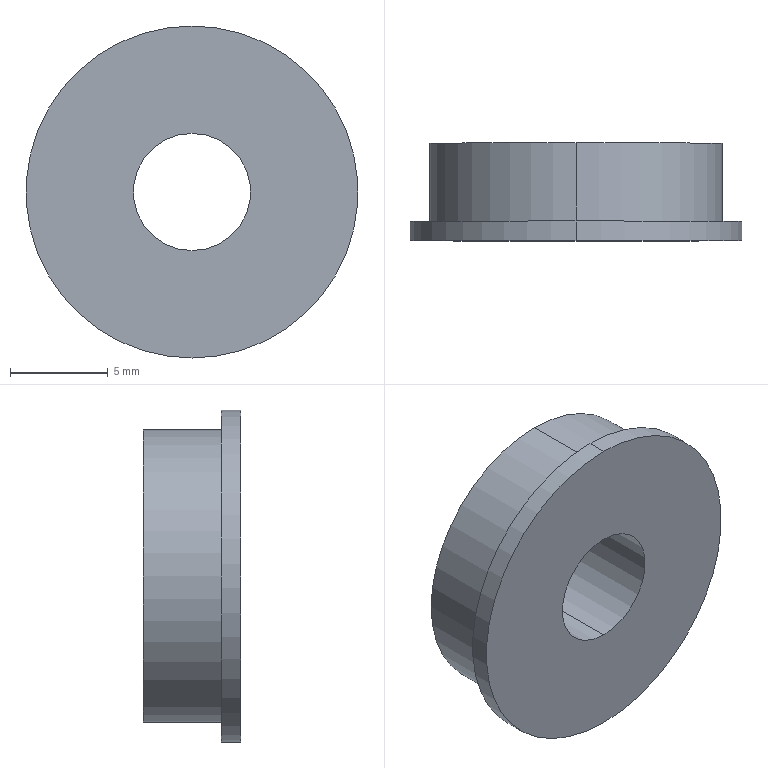Part | SolidWorks | features Revolution 1 | 1 solid | 9 faces | box 17 x 5 x 17 mm | volume 792.467 mm3 | cylinder 6 | plane 3 | commonest cylinder face diameters 6 x2 15 x2 17 x2
STEP:
#1=CARTESIAN_POINT('',(0.,-1.683,-8.5));
#2=VERTEX_POINT('',#1);
#3=CARTESIAN_POINT('',(0.,-1.683,8.5));
#4=VERTEX_POINT('',#3);
#5=CARTESIAN_POINT('',(0.,-1.683,0.));
#6=DIRECTION('',(0.,-1.,0.));
#7=DIRECTION('',(0.,0.,-1.));
#8=AXIS2_PLACEMENT_3D('',#5,#6,#7);
#9=CIRCLE('',#8,8.5);
#10=EDGE_CURVE('',#2,#4,#9,.T.);
#11=ORIENTED_EDGE('',*,*,#10,.T.);
#12=CARTESIAN_POINT('',(0.,-2.683,8.5));
#13=VERTEX_POINT('',#12);
#14=CARTESIAN_POINT('',(0.,0.,8.5));
#15=DIRECTION('',(0.,-1.,0.));
#16=VECTOR('',#15,1000.);
#17=LINE('',#14,#16);
#18=EDGE_CURVE('',#4,#13,#17,.T.);
#19=ORIENTED_EDGE('',*,*,#18,.T.);
#20=CARTESIAN_POINT('',(0.,-2.683,-8.5));
#21=VERTEX_POINT('',#20);
#22=CARTESIAN_POINT('',(0.,-2.683,0.));
#23=DIRECTION('',(0.,-1.,0.));
#24=DIRECTION('',(0.,0.,-1.));
#25=AXIS2_PLACEMENT_3D('',#22,#23,#24);
#26=CIRCLE('',#25,8.5);
#27=EDGE_CURVE('',#21,#13,#26,.T.);
#28=ORIENTED_EDGE('',*,*,#27,.F.);
#29=CARTESIAN_POINT('',(0.,0.,-8.5));
#30=DIRECTION('',(0.,-1.,0.));
#31=VECTOR('',#30,1000.);
#32=LINE('',#29,#31);
#33=EDGE_CURVE('',#2,#21,#32,.T.);
#34=ORIENTED_EDGE('',*,*,#33,.F.);
#35=EDGE_LOOP('',(#11,#19,#28,#34));
#36=FACE_OUTER_BOUND('',#35,.T.);
#37=CARTESIAN_POINT('',(0.,0.,0.));
#38=DIRECTION('',(0.,-1.,0.));
#39=DIRECTION('',(0.,0.,-1.));
#40=AXIS2_PLACEMENT_3D('',#37,#38,#39);
#41=CYLINDRICAL_SURFACE('',#40,8.5);
#42=ADVANCED_FACE('',(#36),#41,.T.);
#43=CARTESIAN_POINT('',(0.,2.317,-7.5));
#44=VERTEX_POINT('',#43);
#45=CARTESIAN_POINT('',(0.,2.317,7.5));
#46=VERTEX_POINT('',#45);
#47=CARTESIAN_POINT('',(0.,2.317,0.));
#48=DIRECTION('',(0.,-1.,0.));
#49=DIRECTION('',(0.,0.,-1.));
#50=AXIS2_PLACEMENT_3D('',#47,#48,#49);
#51=CIRCLE('',#50,7.5);
#52=EDGE_CURVE('',#44,#46,#51,.T.);
#53=ORIENTED_EDGE('',*,*,#52,.T.);
#54=CARTESIAN_POINT('',(0.,-1.683,7.5));
#55=VERTEX_POINT('',#54);
#56=CARTESIAN_POINT('',(0.,0.,7.5));
#57=DIRECTION('',(0.,-1.,0.));
#58=VECTOR('',#57,1000.);
#59=LINE('',#56,#58);
#60=EDGE_CURVE('',#46,#55,#59,.T.);
#61=ORIENTED_EDGE('',*,*,#60,.T.);
#62=CARTESIAN_POINT('',(0.,-1.683,-7.5));
#63=VERTEX_POINT('',#62);
#64=CARTESIAN_POINT('',(0.,-1.683,0.));
#65=DIRECTION('',(0.,-1.,0.));
#66=DIRECTION('',(0.,0.,-1.));
#67=AXIS2_PLACEMENT_3D('',#64,#65,#66);
#68=CIRCLE('',#67,7.5);
#69=EDGE_CURVE('',#63,#55,#68,.T.);
#70=ORIENTED_EDGE('',*,*,#69,.F.);
#71=CARTESIAN_POINT('',(0.,0.,-7.5));
#72=DIRECTION('',(0.,-1.,0.));
#73=VECTOR('',#72,1000.);
#74=LINE('',#71,#73);
#75=EDGE_CURVE('',#44,#63,#74,.T.);
#76=ORIENTED_EDGE('',*,*,#75,.F.);
#77=EDGE_LOOP('',(#53,#61,#70,#76));
#78=FACE_OUTER_BOUND('',#77,.T.);
#79=CARTESIAN_POINT('',(0.,0.,0.));
#80=DIRECTION('',(0.,-1.,0.));
#81=DIRECTION('',(0.,0.,-1.));
#82=AXIS2_PLACEMENT_3D('',#79,#80,#81);
#83=CYLINDRICAL_SURFACE('',#82,7.5);
#84=ADVANCED_FACE('',(#78),#83,.T.);
#85=CARTESIAN_POINT('',(0.,2.317,3.));
#86=VERTEX_POINT('',#85);
#87=CARTESIAN_POINT('',(0.,2.317,-3.));
#88=VERTEX_POINT('',#87);
#89=CARTESIAN_POINT('',(0.,2.317,0.));
#90=DIRECTION('',(0.,-1.,0.));
#91=DIRECTION('',(0.,0.,-1.));
#92=AXIS2_PLACEMENT_3D('',#89,#90,#91);
#93=CIRCLE('',#92,3.);
#94=EDGE_CURVE('',#86,#88,#93,.T.);
#95=ORIENTED_EDGE('',*,*,#94,.F.);
#96=CARTESIAN_POINT('',(0.,-2.683,3.));
#97=VERTEX_POINT('',#96);
#98=CARTESIAN_POINT('',(0.,0.,3.));
#99=DIRECTION('',(0.,-1.,0.));
#100=VECTOR('',#99,1000.);
#101=LINE('',#98,#100);
#102=EDGE_CURVE('',#86,#97,#101,.T.);
#103=ORIENTED_EDGE('',*,*,#102,.T.);
#104=CARTESIAN_POINT('',(0.,-2.683,-3.));
#105=VERTEX_POINT('',#104);
#106=CARTESIAN_POINT('',(0.,-2.683,0.));
#107=DIRECTION('',(0.,-1.,0.));
#108=DIRECTION('',(0.,0.,-1.));
#109=AXIS2_PLACEMENT_3D('',#106,#107,#108);
#110=CIRCLE('',#109,3.);
#111=EDGE_CURVE('',#97,#105,#110,.T.);
#112=ORIENTED_EDGE('',*,*,#111,.T.);
#113=CARTESIAN_POINT('',(0.,0.,-3.));
#114=DIRECTION('',(0.,-1.,0.));
#115=VECTOR('',#114,1000.);
#116=LINE('',#113,#115);
#117=EDGE_CURVE('',#88,#105,#116,.T.);
#118=ORIENTED_EDGE('',*,*,#117,.F.);
#119=EDGE_LOOP('',(#95,#103,#112,#118));
#120=FACE_OUTER_BOUND('',#119,.T.);
#121=CARTESIAN_POINT('',(0.,0.,0.));
#122=DIRECTION('',(0.,-1.,0.));
#123=DIRECTION('',(0.,0.,-1.));
#124=AXIS2_PLACEMENT_3D('',#121,#122,#123);
#125=CYLINDRICAL_SURFACE('',#124,3.);
#126=ADVANCED_FACE('',(#120),#125,.F.);
#127=ORIENTED_EDGE('',*,*,#102,.F.);
#128=CARTESIAN_POINT('',(0.,2.317,0.));
#129=DIRECTION('',(0.,-1.,0.));
#130=DIRECTION('',(0.,0.,-1.));
#131=AXIS2_PLACEMENT_3D('',#128,#129,#130);
#132=CIRCLE('',#131,3.);
#133=EDGE_CURVE('',#88,#86,#132,.T.);
#134=ORIENTED_EDGE('',*,*,#133,.F.);
#135=ORIENTED_EDGE('',*,*,#117,.T.);
#136=CARTESIAN_POINT('',(0.,-2.683,0.));
#137=DIRECTION('',(0.,-1.,0.));
#138=DIRECTION('',(0.,0.,-1.));
#139=AXIS2_PLACEMENT_3D('',#136,#137,#138);
#140=CIRCLE('',#139,3.);
#141=EDGE_CURVE('',#105,#97,#140,.T.);
#142=ORIENTED_EDGE('',*,*,#141,.T.);
#143=EDGE_LOOP('',(#127,#134,#135,#142));
#144=FACE_OUTER_BOUND('',#143,.T.);
#145=CARTESIAN_POINT('',(0.,0.,0.));
#146=DIRECTION('',(0.,-1.,0.));
#147=DIRECTION('',(0.,0.,-1.));
#148=AXIS2_PLACEMENT_3D('',#145,#146,#147);
#149=CYLINDRICAL_SURFACE('',#148,3.);
#150=ADVANCED_FACE('',(#144),#149,.F.);
#151=ORIENTED_EDGE('',*,*,#133,.T.);
#152=ORIENTED_EDGE('',*,*,#94,.T.);
#153=EDGE_LOOP('',(#151,#152));
#154=FACE_BOUND('',#153,.T.);
#155=ORIENTED_EDGE('',*,*,#52,.F.);
#156=CARTESIAN_POINT('',(0.,2.317,0.));
#157=DIRECTION('',(0.,-1.,0.));
#158=DIRECTION('',(0.,0.,-1.));
#159=AXIS2_PLACEMENT_3D('',#156,#157,#158);
#160=CIRCLE('',#159,7.5);
#161=EDGE_CURVE('',#46,#44,#160,.T.);
#162=ORIENTED_EDGE('',*,*,#161,.F.);
#163=EDGE_LOOP('',(#155,#162));
#164=FACE_OUTER_BOUND('',#163,.T.);
#165=CARTESIAN_POINT('',(3.,2.317,0.));
#166=DIRECTION('',(0.,1.,0.));
#167=DIRECTION('',(0.,0.,1.));
#168=AXIS2_PLACEMENT_3D('',#165,#166,#167);
#169=PLANE('',#168);
#170=ADVANCED_FACE('',(#154,#164),#169,.T.);
#171=ORIENTED_EDGE('',*,*,#60,.F.);
#172=ORIENTED_EDGE('',*,*,#161,.T.);
#173=ORIENTED_EDGE('',*,*,#75,.T.);
#174=CARTESIAN_POINT('',(0.,-1.683,0.));
#175=DIRECTION('',(0.,-1.,0.));
#176=DIRECTION('',(0.,0.,-1.));
#177=AXIS2_PLACEMENT_3D('',#174,#175,#176);
#178=CIRCLE('',#177,7.5);
#179=EDGE_CURVE('',#55,#63,#178,.T.);
#180=ORIENTED_EDGE('',*,*,#179,.F.);
#181=EDGE_LOOP('',(#171,#172,#173,#180));
#182=FACE_OUTER_BOUND('',#181,.T.);
#183=CARTESIAN_POINT('',(0.,0.,0.));
#184=DIRECTION('',(0.,-1.,0.));
#185=DIRECTION('',(0.,0.,-1.));
#186=AXIS2_PLACEMENT_3D('',#183,#184,#185);
#187=CYLINDRICAL_SURFACE('',#186,7.5);
#188=ADVANCED_FACE('',(#182),#187,.T.);
#189=ORIENTED_EDGE('',*,*,#69,.T.);
#190=ORIENTED_EDGE('',*,*,#179,.T.);
#191=EDGE_LOOP('',(#189,#190));
#192=FACE_BOUND('',#191,.T.);
#193=ORIENTED_EDGE('',*,*,#10,.F.);
#194=CARTESIAN_POINT('',(0.,-1.683,0.));
#195=DIRECTION('',(0.,-1.,0.));
#196=DIRECTION('',(0.,0.,-1.));
#197=AXIS2_PLACEMENT_3D('',#194,#195,#196);
#198=CIRCLE('',#197,8.5);
#199=EDGE_CURVE('',#4,#2,#198,.T.);
#200=ORIENTED_EDGE('',*,*,#199,.F.);
#201=EDGE_LOOP('',(#193,#200));
#202=FACE_OUTER_BOUND('',#201,.T.);
#203=CARTESIAN_POINT('',(7.5,-1.683,0.));
#204=DIRECTION('',(0.,1.,0.));
#205=DIRECTION('',(0.,0.,1.));
#206=AXIS2_PLACEMENT_3D('',#203,#204,#205);
#207=PLANE('',#206);
#208=ADVANCED_FACE('',(#192,#202),#207,.T.);
#209=ORIENTED_EDGE('',*,*,#18,.F.);
#210=ORIENTED_EDGE('',*,*,#199,.T.);
#211=ORIENTED_EDGE('',*,*,#33,.T.);
#212=CARTESIAN_POINT('',(0.,-2.683,0.));
#213=DIRECTION('',(0.,-1.,0.));
#214=DIRECTION('',(0.,0.,-1.));
#215=AXIS2_PLACEMENT_3D('',#212,#213,#214);
#216=CIRCLE('',#215,8.5);
#217=EDGE_CURVE('',#13,#21,#216,.T.);
#218=ORIENTED_EDGE('',*,*,#217,.F.);
#219=EDGE_LOOP('',(#209,#210,#211,#218));
#220=FACE_OUTER_BOUND('',#219,.T.);
#221=CARTESIAN_POINT('',(0.,0.,0.));
#222=DIRECTION('',(0.,-1.,0.));
#223=DIRECTION('',(0.,0.,-1.));
#224=AXIS2_PLACEMENT_3D('',#221,#222,#223);
#225=CYLINDRICAL_SURFACE('',#224,8.5);
#226=ADVANCED_FACE('',(#220),#225,.T.);
#227=ORIENTED_EDGE('',*,*,#27,.T.);
#228=ORIENTED_EDGE('',*,*,#217,.T.);
#229=EDGE_LOOP('',(#227,#228));
#230=FACE_OUTER_BOUND('',#229,.T.);
#231=ORIENTED_EDGE('',*,*,#141,.F.);
#232=ORIENTED_EDGE('',*,*,#111,.F.);
#233=EDGE_LOOP('',(#231,#232));
#234=FACE_BOUND('',#233,.T.);
#235=CARTESIAN_POINT('',(8.5,-2.683,0.));
#236=DIRECTION('',(0.,-1.,0.));
#237=DIRECTION('',(0.,0.,-1.));
#238=AXIS2_PLACEMENT_3D('',#235,#236,#237);
#239=PLANE('',#238);
#240=ADVANCED_FACE('',(#230,#234),#239,.T.);
#241=CLOSED_SHELL('',(#42,#84,#126,#150,#170,#188,#208,#226,#240));
#242=MANIFOLD_SOLID_BREP('',#241);
#243=CARTESIAN_POINT('',(0.,0.,0.));
#244=DIRECTION('',(0.,0.,1.));
#245=DIRECTION('',(1.,0.,0.));
#246=AXIS2_PLACEMENT_3D('',#243,#244,#245);
#247=(LENGTH_UNIT()NAMED_UNIT(*)SI_UNIT(.MILLI.,.METRE.));
#248=UNCERTAINTY_MEASURE_WITH_UNIT(LENGTH_MEASURE(0.00001),#247,'','');
#249=(NAMED_UNIT(*)PLANE_ANGLE_UNIT()SI_UNIT($,.RADIAN.));
#250=(NAMED_UNIT(*)SI_UNIT($,.STERADIAN.)SOLID_ANGLE_UNIT());
#251=(GEOMETRIC_REPRESENTATION_CONTEXT(3)GLOBAL_UNCERTAINTY_ASSIGNED_CONTEXT((#248))GLOBAL_UNIT_ASSIGNED_CONTEXT((#247,#249,#250))REPRESENTATION_CONTEXT('',''));
#252=ADVANCED_BREP_SHAPE_REPRESENTATION('',(#242,#246),#251);